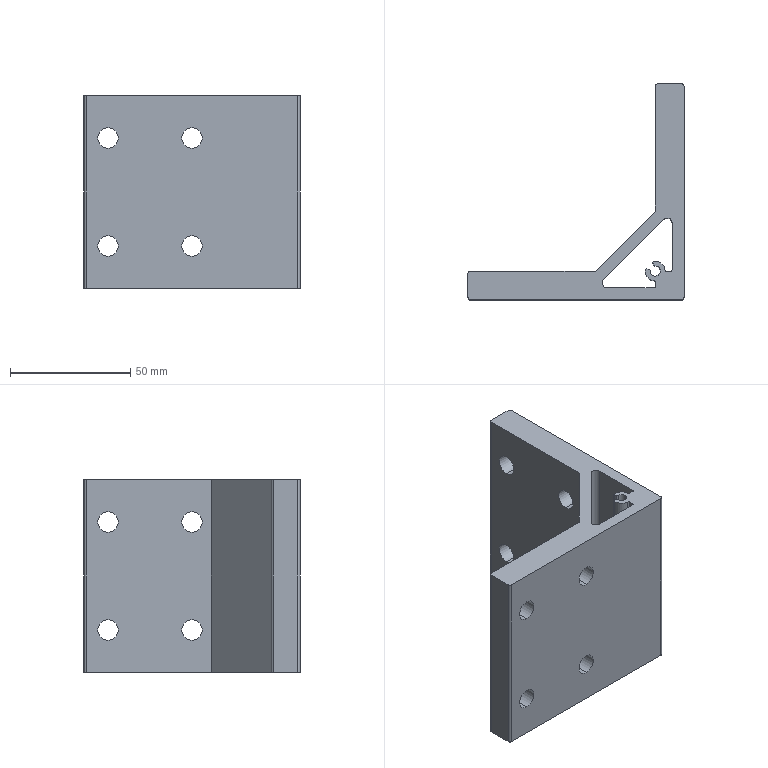Part | STEP file | 001-010-ABC01-4510-90-80 | 1 solid | 53 faces | box 90 x 90 x 80 mm | volume 146220 mm3 | cylinder 37 | plane 16 | commonest cylinder face diameters 8.5 x16 1 x9 2 x5 4.2 x3 4 x2 8.2 x2